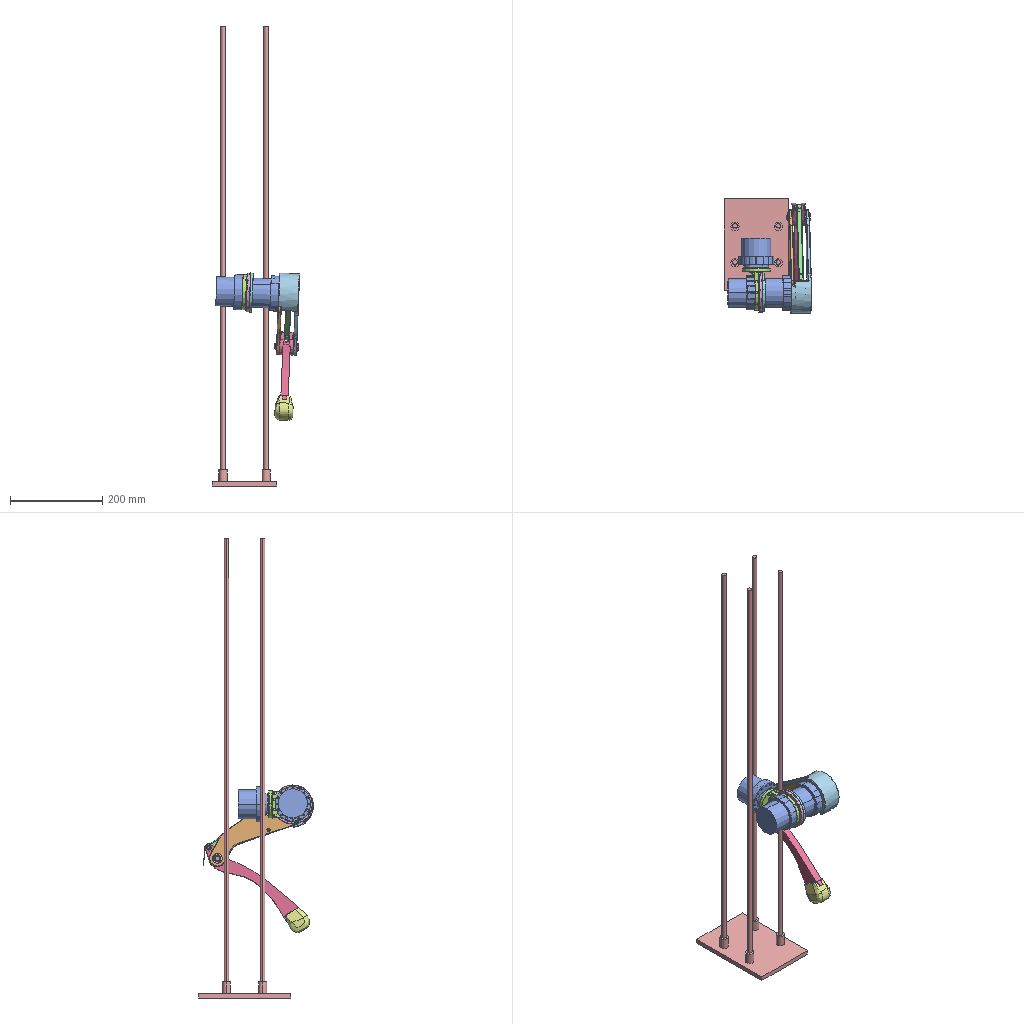Assembly | SolidWorks | 31 different items | 41 placed | box 190 x 250 x 1000 mm
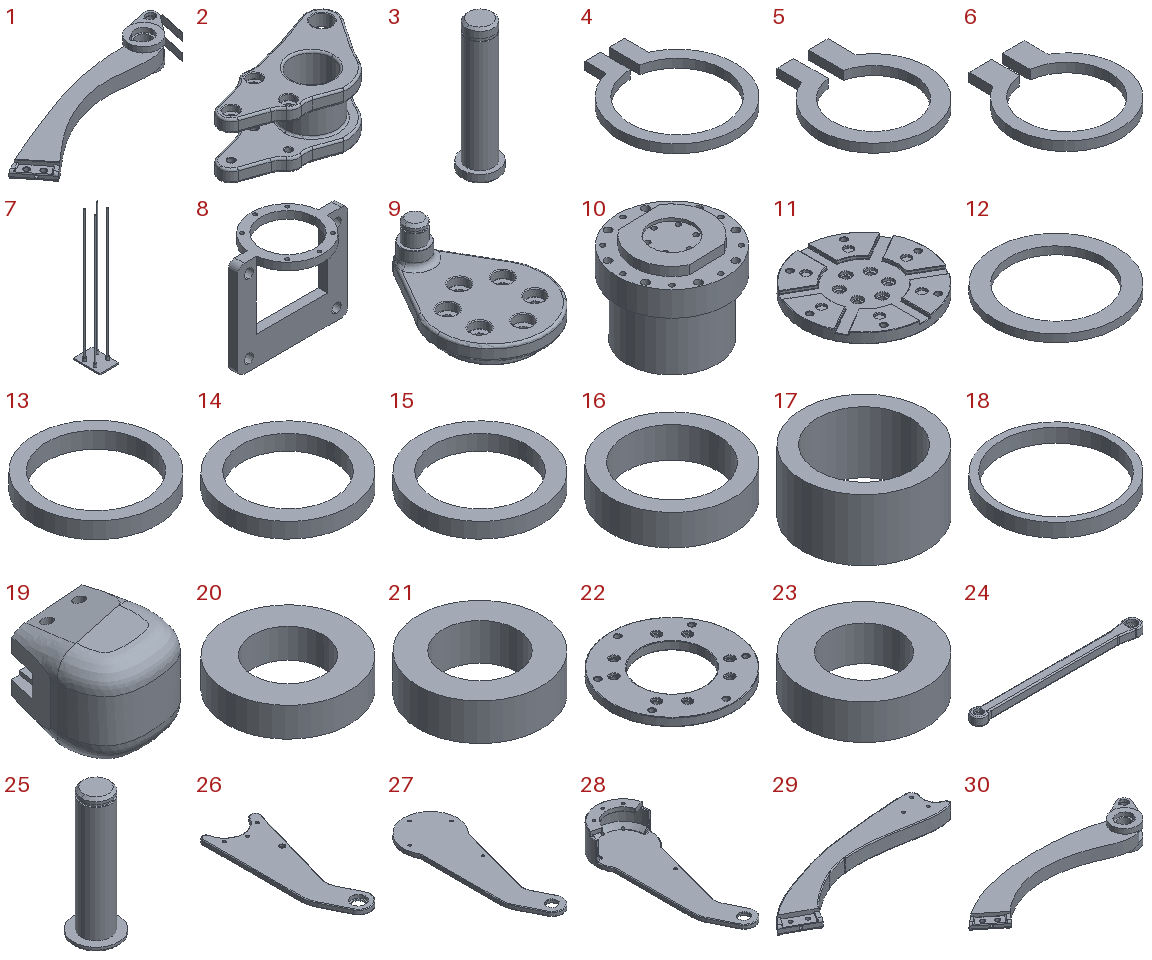Parts list (item | quantity | size | volume | features):
1 | x1 | 245.132 x 107.958 x 30 mm | 99502 mm3 | features ICE 18, Fillet 5, Extrusion 1, MirrorPattern 1
2 | x1 | 77.714 x 44.619 x 29 mm | 22578 mm3 | features ICE 7, Fillet 6, Extrusion 1, MirrorPattern 1
3 | x1 | 8 x 8 x 29.5 mm | 858.581 mm3 | features ICE 3, Chamfer 1, Extrusion 1
4 | x1 | 13.6 x 15.815 x 1 mm | 57.5 mm3 | features Extrusion 1
5 | x1 | 7.6 x 8.962 x 0.6 mm | 14.197 mm3 | features Extrusion 1
6 | x1 | 9.38 x 10.788 x 0.8 mm | 25.334 mm3 | features Extrusion 1
7 | x1 | 140 x 200 x 1000 mm | 608611 mm3 | features ICE 2, Extrusion 1
8 | x1 | 118 x 77 x 103 mm | 78200 mm3 | features ICE 4, Extrusion 1, Fillet 1
9 | x1 | 42 x 57 x 23.6 mm | 12622 mm3 | features ICE 7, Fillet 4, Chamfer 1, Extrusion 1
10 | x3 | 76.5 x 76.5 x 63 mm | 212682 mm3 | features ICE 3, Extrusion 1
11 | x1 | 85 x 85 x 12.3 mm | 37399 mm3 | features ICE 7, Fillet 2, Extrusion 1
12 | x2 | 16 x 16 x 1 mm | 87.965 mm3 | features Extrusion 1
13 | x2 | 15 x 15 x 2 mm | 127.235 mm3 | features Extrusion 1
14 | x1 | 16 x 16 x 2 mm | 175.929 mm3 | features Extrusion 1
15 | x1 | 8 x 8 x 1 mm | 21.991 mm3 | features Extrusion 1
16 | x1 | 8 x 8 x 2 mm | 43.982 mm3 | features Extrusion 1
17 | x1 | 8 x 8 x 4 mm | 87.965 mm3 | features Extrusion 1
18 | x1 | 9 x 9 x 1 mm | 13.352 mm3 | features Extrusion 1
19 | x1 | 44.726 x 47.714 x 39 mm | 59211 mm3 | features ICE 6, Extrusion 1, Fillet 1, MirrorPattern 1
20 | x4 | 21 x 21 x 5 mm | 1166 mm3 | features Extrusion 1
21 | x4 | 10 x 10 x 3 mm | 150.796 mm3 | features Extrusion 1
22 | x1 | 85 x 85 x 5.5 mm | 21445 mm3 | features ICE 3, Fillet 2, Extrusion 1
23 | x1 | 14 x 14 x 4 mm | 414.69 mm3 | features Extrusion 1
24 | x1 | 219 x 20 x 11 mm | 26143 mm3 | features ICE 10, Fillet 2, Extrusion 1
25 | x1 | 18 x 18 x 51 mm | 5715 mm3 | features ICE 3, Chamfer 1, Extrusion 1
26 | x1 | 76.423 x 217.462 x 7 mm | 66603 mm3 | features Fillet 5, ICE 4, Extrusion 1
27 | x1 | 88 x 261.5 x 7 mm | 97457 mm3 | features Fillet 5, ICE 3, Extrusion 1
28 | x1 | 90 x 262.5 x 44 mm | 128992 mm3 | features ICE 8, Fillet 4, Chamfer 1, Extrusion 1
29 | x1 | 223.949 x 75.75 x 16 mm | 90411 mm3 | features ICE 7, Fillet 4, Extrusion 1, MirrorPattern 1
30 | x1 | 253.853 x 64.863 x 29 mm | 119794 mm3 | features ICE 16, Fillet 5, Extrusion 1, MirrorPattern 1
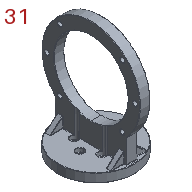31 | x1 | 60 x 77 x 95.8 mm | 43529 mm3 | features ICE 6, Fillet 2, Extrusion 1, MirrorPattern 1
Mates (type | each side: item.copy, entity, surface, feature):
Concentric | 7.1 face cylinder Boss-Extrude3 | 8.1 face cylinder Cut-Extrude1 | 2 times
Concentric | 8.1 face cylinder Boss-Extrude1 | 10.1 face cylinder Boss-Extrude2 | 2 times
Coincident | 8.1 face plane Boss-Extrude1 | 10.1 face plane Boss-Extrude2
Concentric | 10.1 face cylinder Cut-Extrude1 | 31.1 face cylinder Boss-Extrude2
Coincident | 10.1 face plane Cut-Extrude1 | 31.1 face plane Boss-Extrude2
Concentric | 31.1 face cylinder Boss-Extrude4 | 10.2 face cylinder Boss-Extrude2 | 2 times
Coincident | 31.1 face plane Boss-Extrude4 | 10.2 face plane Boss-Extrude2
Concentric | 10.2 face cylinder Cut-Extrude1 | 11.1 face cylinder Boss-Extrude2
Coincident | 10.2 face plane Cut-Extrude1 | 11.1 face plane Boss-Extrude2
Concentric | 11.1 face cylinder Cut-Extrude8 | 22.1 face cylinder Cut-Extrude1 | 2 times
Coincident | 11.1 face plane Boss-Extrude1 | 22.1 face plane Boss-Extrude1
Concentric | 22.1 face cylinder Boss-Extrude1 | 10.3 face cylinder Boss-Extrude3
Coincident | 22.1 face plane Boss-Extrude1 | 10.3 face plane Boss-Extrude3
Concentric | 10.3 face cylinder Boss-Extrude2 | 26.1 face cylinder Boss-Extrude1
Concentric | 10.3 edge | 26.1 face cylinder Boss-Extrude1
Coincident | 10.3 face plane Boss-Extrude2 | 26.1 face plane Boss-Extrude1
Concentric | 10.3 face cylinder Cut-Extrude1 | 9.1 face cylinder Boss-Extrude2
Coincident | 10.3 face plane Cut-Extrude1 | 9.1 face plane Boss-Extrude2
Concentric | 9.1 face cylinder Boss-Extrude4 | 24.1 face cylinder Boss-Extrude1
Coincident | 9.1 face plane Boss-Extrude3 | 24.1 face plane Cut-Extrude3
Concentric | 26.1 face cylinder Cut-Extrude1 | 1.1 face cylinder Boss-Extrude1
Concentric | 24.1 face cylinder Boss-Extrude1 | 1.1 face cylinder Mirror3
Concentric | 10.3 face cylinder Boss-Extrude2 | 28.1 face cylinder Cut-Extrude6 | 2 times
Coincident | 10.3 face plane Boss-Extrude2 | 28.1 face plane Boss-Extrude4
Parallel | 26.1 face cylinder Boss-Extrude1 | 1.1 face surface:4009 Boss-Extrude3
Coincident | 1.1 face plane Mirror3 | 19.1 face plane Cut-Extrude2
Concentric | 1.1 face cylinder Cut-Extrude3 | 19.1 face cylinder Cut-Extrude6 | 2 times
Concentric | 9.1 face cylinder Boss-Extrude4 | 23.1 face cylinder Boss-Extrude1
Coincident | 9.1 face plane Boss-Extrude3 | 23.1 face plane Boss-Extrude1
Concentric | 1.1 face cylinder Cut-Extrude5 | 21.1 face cylinder Boss-Extrude1
Concentric | 1.1 face cylinder Mirror3 | 21.2 face cylinder Boss-Extrude1
Coincident | 1.1 face plane Cut-Extrude9 | 21.2 face plane Boss-Extrude1
Concentric | 24.1 face cylinder Cut-Extrude9 | 21.3 face cylinder Boss-Extrude1
Concentric | 24.1 face cylinder Cut-Extrude10 | 21.4 face cylinder Boss-Extrude1
Coincident | 24.1 face plane Cut-Extrude1 | 21.4 edge
Coincident | 24.1 face plane Cut-Extrude6 | 21.3 face plane Boss-Extrude1
Concentric | 21.1 face cylinder Boss-Extrude1 | 3.1 face cylinder Boss-Extrude2
Concentric | 3.1 face cylinder Boss-Extrude4 | 15.1 face cylinder Boss-Extrude1
Coincident | 21.2 face plane Boss-Extrude1 | 15.1 face plane Boss-Extrude1
Coincident | 21.1 face plane Boss-Extrude1 | 3.1 face plane Boss-Extrude1
Concentric | 1.1 face cylinder Boss-Extrude1 | 20.1 face cylinder Boss-Extrude1
Coincident | 1.1 face plane Cut-Extrude13 | 20.1 face plane Boss-Extrude1
Concentric | 1.1 face cylinder Boss-Extrude1 | 20.2 face cylinder Boss-Extrude1
Coincident | 1.1 face plane Cut-Extrude14 | 20.2 face plane Boss-Extrude1
Concentric | 28.1 face cylinder Cut-Extrude1 | 20.3 face cylinder Boss-Extrude1
Coincident | 28.1 face plane Boss-Extrude1 | 20.3 face plane Boss-Extrude1
Concentric | 26.1 face cylinder Cut-Extrude1 | 20.4 face cylinder Boss-Extrude1
Coincident | 26.1 face plane Boss-Extrude1 | 20.4 face plane Boss-Extrude1
Concentric | 20.3 face cylinder Boss-Extrude1 | 25.1 face cylinder Boss-Extrude2
Concentric | 25.1 face cylinder Boss-Extrude2 | 12.1 face cylinder Boss-Extrude1
Coincident | 20.3 face plane Boss-Extrude1 | 12.1 face plane Boss-Extrude1
Coincident | 25.1 face plane Boss-Extrude1 | 12.1 face plane Boss-Extrude1
Concentric | 25.1 face cylinder Boss-Extrude2 | 12.2 face cylinder Boss-Extrude1
Coincident | 20.4 face plane Boss-Extrude1 | 12.2 face plane Boss-Extrude1
Concentric | 25.1 face cylinder Boss-Extrude3 | 4.1 face cylinder Boss-Extrude1
Coincident | 12.2 face plane Boss-Extrude1 | 4.1 face plane Boss-Extrude1
Concentric | 3.1 face cylinder Boss-Extrude3 | 5.1 face cylinder Boss-Extrude1
Coincident | 3.1 face plane Boss-Extrude2 | 5.1 face plane Boss-Extrude1
Concentric | 9.1 face cylinder Boss-Extrude5 | 6.1 face cylinder Boss-Extrude1
Concentric | 9.1 face cylinder Boss-Extrude5 | 18.1 face cylinder Boss-Extrude1
Coincident | 23.1 face plane Boss-Extrude1 | 18.1 face plane Boss-Extrude1
Coincident | 9.1 face plane Boss-Extrude4 | 6.1 face plane Boss-Extrude1
Concentric | 3.1 face cylinder Boss-Extrude2 | 17.1 face cylinder Boss-Extrude1
Coincident | 21.3 face plane Boss-Extrude1 | 17.1 face plane Boss-Extrude1
Coincident | 1.1 face plane Cut-Extrude5 | 21.1 face plane Boss-Extrude1
Concentric | 3.1 face cylinder Boss-Extrude2 | 16.1 face cylinder Boss-Extrude1
Coincident | 21.4 face plane Boss-Extrude1 | 16.1 face plane Boss-Extrude1
Concentric | 25.1 face cylinder Boss-Extrude2 | 13.1 face cylinder Boss-Extrude1
Coincident | 20.1 face plane Boss-Extrude1 | 13.1 face plane Boss-Extrude1
Concentric | 25.1 face cylinder Boss-Extrude2 | 13.2 face cylinder Boss-Extrude1
Coincident | 20.4 face plane Boss-Extrude1 | 13.2 face plane Boss-Extrude1
DistanceDim | 1.1 face plane Cut-Extrude14 | 26.1 face plane Boss-Extrude1